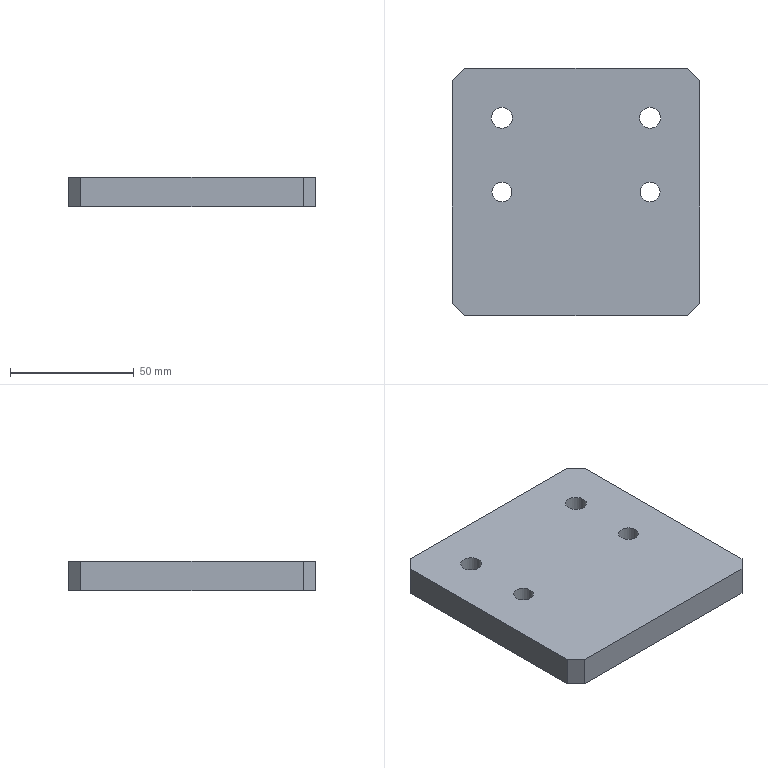Part | NX | features BREP 1 | 1 solid | 14 faces | box 100 x 100 x 12 mm | volume 116832 mm3 | plane 10 | cylinder 4 | commonest cylinder face diameters 8 x2 8.5 x2
STEP:
#1=CARTESIAN_POINT('',(50.,45.,3.));
#2=VERTEX_POINT('',#1);
#3=CARTESIAN_POINT('',(50.,-45.,3.));
#4=VERTEX_POINT('',#3);
#5=CARTESIAN_POINT('',(50.,50.,3.));
#6=DIRECTION('',(0.,-1.,0.));
#7=VECTOR('',#6,1000.);
#8=LINE('',#5,#7);
#9=EDGE_CURVE('',#2,#4,#8,.T.);
#10=ORIENTED_EDGE('',*,*,#9,.F.);
#11=CARTESIAN_POINT('',(50.,45.,15.));
#12=VERTEX_POINT('',#11);
#13=CARTESIAN_POINT('',(50.,45.,15.));
#14=DIRECTION('',(0.,0.,1.));
#15=VECTOR('',#14,1000.);
#16=LINE('',#13,#15);
#17=EDGE_CURVE('',#2,#12,#16,.T.);
#18=ORIENTED_EDGE('',*,*,#17,.T.);
#19=CARTESIAN_POINT('',(50.,-45.,15.));
#20=VERTEX_POINT('',#19);
#21=CARTESIAN_POINT('',(50.,50.,15.));
#22=DIRECTION('',(0.,1.,0.));
#23=VECTOR('',#22,1000.);
#24=LINE('',#21,#23);
#25=EDGE_CURVE('',#20,#12,#24,.T.);
#26=ORIENTED_EDGE('',*,*,#25,.F.);
#27=CARTESIAN_POINT('',(50.,-45.,15.));
#28=DIRECTION('',(0.,0.,-1.));
#29=VECTOR('',#28,1000.);
#30=LINE('',#27,#29);
#31=EDGE_CURVE('',#20,#4,#30,.T.);
#32=ORIENTED_EDGE('',*,*,#31,.T.);
#33=EDGE_LOOP('',(#10,#18,#26,#32));
#34=FACE_BOUND('',#33,.T.);
#35=CARTESIAN_POINT('',(50.,50.,15.));
#36=DIRECTION('',(-1.,0.,0.));
#37=DIRECTION('',(0.,0.,-1.));
#38=AXIS2_PLACEMENT_3D('',#35,#36,#37);
#39=PLANE('',#38);
#40=ADVANCED_FACE('',(#34),#39,.F.);
#41=CARTESIAN_POINT('',(45.,50.,3.));
#42=VERTEX_POINT('',#41);
#43=CARTESIAN_POINT('',(-45.,50.,3.));
#44=VERTEX_POINT('',#43);
#45=CARTESIAN_POINT('',(570.,50.,3.));
#46=DIRECTION('',(-1.,0.,0.));
#47=VECTOR('',#46,1000.);
#48=LINE('',#45,#47);
#49=EDGE_CURVE('',#42,#44,#48,.T.);
#50=ORIENTED_EDGE('',*,*,#49,.T.);
#51=CARTESIAN_POINT('',(-45.,50.,15.));
#52=VERTEX_POINT('',#51);
#53=CARTESIAN_POINT('',(-45.,50.,15.));
#54=DIRECTION('',(0.,0.,1.));
#55=VECTOR('',#54,1000.);
#56=LINE('',#53,#55);
#57=EDGE_CURVE('',#44,#52,#56,.T.);
#58=ORIENTED_EDGE('',*,*,#57,.T.);
#59=CARTESIAN_POINT('',(45.,50.,15.));
#60=VERTEX_POINT('',#59);
#61=CARTESIAN_POINT('',(-50.,50.,15.));
#62=DIRECTION('',(-1.,0.,0.));
#63=VECTOR('',#62,1000.);
#64=LINE('',#61,#63);
#65=EDGE_CURVE('',#60,#52,#64,.T.);
#66=ORIENTED_EDGE('',*,*,#65,.F.);
#67=CARTESIAN_POINT('',(45.,50.,15.));
#68=DIRECTION('',(0.,0.,-1.));
#69=VECTOR('',#68,1000.);
#70=LINE('',#67,#69);
#71=EDGE_CURVE('',#60,#42,#70,.T.);
#72=ORIENTED_EDGE('',*,*,#71,.T.);
#73=EDGE_LOOP('',(#50,#58,#66,#72));
#74=FACE_BOUND('',#73,.T.);
#75=CARTESIAN_POINT('',(-50.,50.,15.));
#76=DIRECTION('',(0.,-1.,0.));
#77=DIRECTION('',(0.,0.,1.));
#78=AXIS2_PLACEMENT_3D('',#75,#76,#77);
#79=PLANE('',#78);
#80=ADVANCED_FACE('',(#74),#79,.F.);
#81=CARTESIAN_POINT('',(-50.,-45.,3.));
#82=VERTEX_POINT('',#81);
#83=CARTESIAN_POINT('',(-50.,45.,3.));
#84=VERTEX_POINT('',#83);
#85=CARTESIAN_POINT('',(-50.,50.,3.));
#86=DIRECTION('',(0.,1.,0.));
#87=VECTOR('',#86,1000.);
#88=LINE('',#85,#87);
#89=EDGE_CURVE('',#82,#84,#88,.T.);
#90=ORIENTED_EDGE('',*,*,#89,.F.);
#91=CARTESIAN_POINT('',(-50.,-45.,15.));
#92=VERTEX_POINT('',#91);
#93=CARTESIAN_POINT('',(-50.,-45.,15.));
#94=DIRECTION('',(0.,0.,1.));
#95=VECTOR('',#94,1000.);
#96=LINE('',#93,#95);
#97=EDGE_CURVE('',#82,#92,#96,.T.);
#98=ORIENTED_EDGE('',*,*,#97,.T.);
#99=CARTESIAN_POINT('',(-50.,45.,15.));
#100=VERTEX_POINT('',#99);
#101=CARTESIAN_POINT('',(-50.,50.,15.));
#102=DIRECTION('',(0.,-1.,0.));
#103=VECTOR('',#102,1000.);
#104=LINE('',#101,#103);
#105=EDGE_CURVE('',#100,#92,#104,.T.);
#106=ORIENTED_EDGE('',*,*,#105,.F.);
#107=CARTESIAN_POINT('',(-50.,45.,15.));
#108=DIRECTION('',(0.,0.,-1.));
#109=VECTOR('',#108,1000.);
#110=LINE('',#107,#109);
#111=EDGE_CURVE('',#100,#84,#110,.T.);
#112=ORIENTED_EDGE('',*,*,#111,.T.);
#113=EDGE_LOOP('',(#90,#98,#106,#112));
#114=FACE_BOUND('',#113,.T.);
#115=CARTESIAN_POINT('',(-50.,50.,15.));
#116=DIRECTION('',(1.,0.,0.));
#117=DIRECTION('',(0.,-1.,0.));
#118=AXIS2_PLACEMENT_3D('',#115,#116,#117);
#119=PLANE('',#118);
#120=ADVANCED_FACE('',(#114),#119,.F.);
#121=CARTESIAN_POINT('',(45.,-50.,3.));
#122=VERTEX_POINT('',#121);
#123=CARTESIAN_POINT('',(-45.,-50.,3.));
#124=VERTEX_POINT('',#123);
#125=CARTESIAN_POINT('',(-50.,-50.,3.));
#126=DIRECTION('',(-1.,0.,0.));
#127=VECTOR('',#126,1000.);
#128=LINE('',#125,#127);
#129=EDGE_CURVE('',#122,#124,#128,.T.);
#130=ORIENTED_EDGE('',*,*,#129,.F.);
#131=CARTESIAN_POINT('',(45.,-50.,15.));
#132=VERTEX_POINT('',#131);
#133=CARTESIAN_POINT('',(45.,-50.,15.));
#134=DIRECTION('',(0.,0.,1.));
#135=VECTOR('',#134,1000.);
#136=LINE('',#133,#135);
#137=EDGE_CURVE('',#122,#132,#136,.T.);
#138=ORIENTED_EDGE('',*,*,#137,.T.);
#139=CARTESIAN_POINT('',(-45.,-50.,15.));
#140=VERTEX_POINT('',#139);
#141=CARTESIAN_POINT('',(-50.,-50.,15.));
#142=DIRECTION('',(1.,0.,0.));
#143=VECTOR('',#142,1000.);
#144=LINE('',#141,#143);
#145=EDGE_CURVE('',#140,#132,#144,.T.);
#146=ORIENTED_EDGE('',*,*,#145,.F.);
#147=CARTESIAN_POINT('',(-45.,-50.,15.));
#148=DIRECTION('',(0.,0.,-1.));
#149=VECTOR('',#148,1000.);
#150=LINE('',#147,#149);
#151=EDGE_CURVE('',#140,#124,#150,.T.);
#152=ORIENTED_EDGE('',*,*,#151,.T.);
#153=EDGE_LOOP('',(#130,#138,#146,#152));
#154=FACE_BOUND('',#153,.T.);
#155=CARTESIAN_POINT('',(-50.,-50.,15.));
#156=DIRECTION('',(0.,1.,0.));
#157=DIRECTION('',(0.,0.,-1.));
#158=AXIS2_PLACEMENT_3D('',#155,#156,#157);
#159=PLANE('',#158);
#160=ADVANCED_FACE('',(#154),#159,.F.);
#161=ORIENTED_EDGE('',*,*,#97,.F.);
#162=CARTESIAN_POINT('',(-45.,-50.,3.));
#163=DIRECTION('',(0.7071,-0.7071,0.));
#164=VECTOR('',#163,1000.);
#165=LINE('',#162,#164);
#166=EDGE_CURVE('',#82,#124,#165,.T.);
#167=ORIENTED_EDGE('',*,*,#166,.T.);
#168=ORIENTED_EDGE('',*,*,#151,.F.);
#169=CARTESIAN_POINT('',(-47.5,-47.5,15.));
#170=DIRECTION('',(0.7071,-0.7071,0.));
#171=VECTOR('',#170,1000.);
#172=LINE('',#169,#171);
#173=EDGE_CURVE('',#92,#140,#172,.T.);
#174=ORIENTED_EDGE('',*,*,#173,.F.);
#175=EDGE_LOOP('',(#161,#167,#168,#174));
#176=FACE_BOUND('',#175,.T.);
#177=CARTESIAN_POINT('',(-45.,-50.,15.));
#178=DIRECTION('',(0.7071,0.7071,0.));
#179=DIRECTION('',(0.,0.,1.));
#180=AXIS2_PLACEMENT_3D('',#177,#178,#179);
#181=PLANE('',#180);
#182=ADVANCED_FACE('',(#176),#181,.F.);
#183=ORIENTED_EDGE('',*,*,#137,.F.);
#184=CARTESIAN_POINT('',(50.,-45.,3.));
#185=DIRECTION('',(0.7071,0.7071,0.));
#186=VECTOR('',#185,1000.);
#187=LINE('',#184,#186);
#188=EDGE_CURVE('',#122,#4,#187,.T.);
#189=ORIENTED_EDGE('',*,*,#188,.T.);
#190=ORIENTED_EDGE('',*,*,#31,.F.);
#191=CARTESIAN_POINT('',(47.5,-47.5,15.));
#192=DIRECTION('',(0.7071,0.7071,0.));
#193=VECTOR('',#192,1000.);
#194=LINE('',#191,#193);
#195=EDGE_CURVE('',#132,#20,#194,.T.);
#196=ORIENTED_EDGE('',*,*,#195,.F.);
#197=EDGE_LOOP('',(#183,#189,#190,#196));
#198=FACE_BOUND('',#197,.T.);
#199=CARTESIAN_POINT('',(50.,-45.,15.));
#200=DIRECTION('',(-0.7071,0.7071,0.));
#201=DIRECTION('',(0.,0.,1.));
#202=AXIS2_PLACEMENT_3D('',#199,#200,#201);
#203=PLANE('',#202);
#204=ADVANCED_FACE('',(#198),#203,.F.);
#205=ORIENTED_EDGE('',*,*,#17,.F.);
#206=CARTESIAN_POINT('',(45.,50.,3.));
#207=DIRECTION('',(-0.7071,0.7071,0.));
#208=VECTOR('',#207,1000.);
#209=LINE('',#206,#208);
#210=EDGE_CURVE('',#2,#42,#209,.T.);
#211=ORIENTED_EDGE('',*,*,#210,.T.);
#212=ORIENTED_EDGE('',*,*,#71,.F.);
#213=CARTESIAN_POINT('',(47.5,47.5,15.));
#214=DIRECTION('',(-0.7071,0.7071,0.));
#215=VECTOR('',#214,1000.);
#216=LINE('',#213,#215);
#217=EDGE_CURVE('',#12,#60,#216,.T.);
#218=ORIENTED_EDGE('',*,*,#217,.F.);
#219=EDGE_LOOP('',(#205,#211,#212,#218));
#220=FACE_BOUND('',#219,.T.);
#221=CARTESIAN_POINT('',(45.,50.,15.));
#222=DIRECTION('',(-0.7071,-0.7071,0.));
#223=DIRECTION('',(0.,0.,1.));
#224=AXIS2_PLACEMENT_3D('',#221,#222,#223);
#225=PLANE('',#224);
#226=ADVANCED_FACE('',(#220),#225,.F.);
#227=ORIENTED_EDGE('',*,*,#57,.F.);
#228=CARTESIAN_POINT('',(-50.,45.,3.));
#229=DIRECTION('',(-0.7071,-0.7071,0.));
#230=VECTOR('',#229,1000.);
#231=LINE('',#228,#230);
#232=EDGE_CURVE('',#44,#84,#231,.T.);
#233=ORIENTED_EDGE('',*,*,#232,.T.);
#234=ORIENTED_EDGE('',*,*,#111,.F.);
#235=CARTESIAN_POINT('',(-47.5,47.5,15.));
#236=DIRECTION('',(-0.7071,-0.7071,0.));
#237=VECTOR('',#236,1000.);
#238=LINE('',#235,#237);
#239=EDGE_CURVE('',#52,#100,#238,.T.);
#240=ORIENTED_EDGE('',*,*,#239,.F.);
#241=EDGE_LOOP('',(#227,#233,#234,#240));
#242=FACE_BOUND('',#241,.T.);
#243=CARTESIAN_POINT('',(-50.,45.,15.));
#244=DIRECTION('',(0.7071,-0.7071,0.));
#245=DIRECTION('',(0.,0.,1.));
#246=AXIS2_PLACEMENT_3D('',#243,#244,#245);
#247=PLANE('',#246);
#248=ADVANCED_FACE('',(#242),#247,.F.);
#249=CARTESIAN_POINT('',(34.25,30.,15.));
#250=VERTEX_POINT('',#249);
#251=CARTESIAN_POINT('',(30.,30.,15.));
#252=DIRECTION('',(0.,0.,1.));
#253=DIRECTION('',(1.,0.,0.));
#254=AXIS2_PLACEMENT_3D('',#251,#252,#253);
#255=CIRCLE('',#254,4.25);
#256=EDGE_CURVE('',#250,#250,#255,.T.);
#257=ORIENTED_EDGE('',*,*,#256,.F.);
#258=EDGE_LOOP('',(#257));
#259=FACE_BOUND('',#258,.T.);
#260=CARTESIAN_POINT('',(-25.75,30.,15.));
#261=VERTEX_POINT('',#260);
#262=CARTESIAN_POINT('',(-30.,30.,15.));
#263=DIRECTION('',(0.,0.,1.));
#264=DIRECTION('',(1.,0.,0.));
#265=AXIS2_PLACEMENT_3D('',#262,#263,#264);
#266=CIRCLE('',#265,4.25);
#267=EDGE_CURVE('',#261,#261,#266,.T.);
#268=ORIENTED_EDGE('',*,*,#267,.F.);
#269=EDGE_LOOP('',(#268));
#270=FACE_BOUND('',#269,.T.);
#271=CARTESIAN_POINT('',(34.,0.,15.));
#272=VERTEX_POINT('',#271);
#273=CARTESIAN_POINT('',(30.,0.,15.));
#274=DIRECTION('',(0.,0.,1.));
#275=DIRECTION('',(1.,0.,0.));
#276=AXIS2_PLACEMENT_3D('',#273,#274,#275);
#277=CIRCLE('',#276,4.);
#278=EDGE_CURVE('',#272,#272,#277,.T.);
#279=ORIENTED_EDGE('',*,*,#278,.F.);
#280=EDGE_LOOP('',(#279));
#281=FACE_BOUND('',#280,.T.);
#282=CARTESIAN_POINT('',(-26.,0.,15.));
#283=VERTEX_POINT('',#282);
#284=CARTESIAN_POINT('',(-30.,0.,15.));
#285=DIRECTION('',(0.,0.,1.));
#286=DIRECTION('',(1.,0.,0.));
#287=AXIS2_PLACEMENT_3D('',#284,#285,#286);
#288=CIRCLE('',#287,4.);
#289=EDGE_CURVE('',#283,#283,#288,.T.);
#290=ORIENTED_EDGE('',*,*,#289,.F.);
#291=EDGE_LOOP('',(#290));
#292=FACE_BOUND('',#291,.T.);
#293=ORIENTED_EDGE('',*,*,#105,.T.);
#294=ORIENTED_EDGE('',*,*,#173,.T.);
#295=ORIENTED_EDGE('',*,*,#145,.T.);
#296=ORIENTED_EDGE('',*,*,#195,.T.);
#297=ORIENTED_EDGE('',*,*,#25,.T.);
#298=ORIENTED_EDGE('',*,*,#217,.T.);
#299=ORIENTED_EDGE('',*,*,#65,.T.);
#300=ORIENTED_EDGE('',*,*,#239,.T.);
#301=EDGE_LOOP('',(#293,#294,#295,#296,#297,#298,#299,#300));
#302=FACE_BOUND('',#301,.T.);
#303=CARTESIAN_POINT('',(0.,0.,15.));
#304=DIRECTION('',(0.,0.,1.));
#305=DIRECTION('',(-1.,0.,0.));
#306=AXIS2_PLACEMENT_3D('',#303,#304,#305);
#307=PLANE('',#306);
#308=ADVANCED_FACE('',(#259,#270,#281,#292,#302),#307,.T.);
#309=CARTESIAN_POINT('',(25.75,30.,3.));
#310=VERTEX_POINT('',#309);
#311=CARTESIAN_POINT('',(30.,30.,3.));
#312=DIRECTION('',(0.,0.,-1.));
#313=DIRECTION('',(-1.,0.,0.));
#314=AXIS2_PLACEMENT_3D('',#311,#312,#313);
#315=CIRCLE('',#314,4.25);
#316=EDGE_CURVE('',#310,#310,#315,.T.);
#317=ORIENTED_EDGE('',*,*,#316,.F.);
#318=EDGE_LOOP('',(#317));
#319=FACE_BOUND('',#318,.T.);
#320=CARTESIAN_POINT('',(-34.25,30.,3.));
#321=VERTEX_POINT('',#320);
#322=CARTESIAN_POINT('',(-30.,30.,3.));
#323=DIRECTION('',(0.,0.,-1.));
#324=DIRECTION('',(-1.,0.,0.));
#325=AXIS2_PLACEMENT_3D('',#322,#323,#324);
#326=CIRCLE('',#325,4.25);
#327=EDGE_CURVE('',#321,#321,#326,.T.);
#328=ORIENTED_EDGE('',*,*,#327,.F.);
#329=EDGE_LOOP('',(#328));
#330=FACE_BOUND('',#329,.T.);
#331=CARTESIAN_POINT('',(26.,0.,3.));
#332=VERTEX_POINT('',#331);
#333=CARTESIAN_POINT('',(30.,0.,3.));
#334=DIRECTION('',(0.,0.,-1.));
#335=DIRECTION('',(-1.,0.,0.));
#336=AXIS2_PLACEMENT_3D('',#333,#334,#335);
#337=CIRCLE('',#336,4.);
#338=EDGE_CURVE('',#332,#332,#337,.T.);
#339=ORIENTED_EDGE('',*,*,#338,.F.);
#340=EDGE_LOOP('',(#339));
#341=FACE_BOUND('',#340,.T.);
#342=CARTESIAN_POINT('',(-34.,0.,3.));
#343=VERTEX_POINT('',#342);
#344=CARTESIAN_POINT('',(-30.,0.,3.));
#345=DIRECTION('',(0.,0.,-1.));
#346=DIRECTION('',(-1.,0.,0.));
#347=AXIS2_PLACEMENT_3D('',#344,#345,#346);
#348=CIRCLE('',#347,4.);
#349=EDGE_CURVE('',#343,#343,#348,.T.);
#350=ORIENTED_EDGE('',*,*,#349,.F.);
#351=EDGE_LOOP('',(#350));
#352=FACE_BOUND('',#351,.T.);
#353=ORIENTED_EDGE('',*,*,#9,.T.);
#354=ORIENTED_EDGE('',*,*,#188,.F.);
#355=ORIENTED_EDGE('',*,*,#129,.T.);
#356=ORIENTED_EDGE('',*,*,#166,.F.);
#357=ORIENTED_EDGE('',*,*,#89,.T.);
#358=ORIENTED_EDGE('',*,*,#232,.F.);
#359=ORIENTED_EDGE('',*,*,#49,.F.);
#360=ORIENTED_EDGE('',*,*,#210,.F.);
#361=EDGE_LOOP('',(#353,#354,#355,#356,#357,#358,#359,#360));
#362=FACE_BOUND('',#361,.T.);
#363=CARTESIAN_POINT('',(-380.,-300.,3.));
#364=DIRECTION('',(0.,0.,-1.));
#365=DIRECTION('',(1.,0.,0.));
#366=AXIS2_PLACEMENT_3D('',#363,#364,#365);
#367=PLANE('',#366);
#368=ADVANCED_FACE('',(#319,#330,#341,#352,#362),#367,.T.);
#369=ORIENTED_EDGE('',*,*,#289,.T.);
#370=EDGE_LOOP('',(#369));
#371=FACE_BOUND('',#370,.T.);
#372=ORIENTED_EDGE('',*,*,#349,.T.);
#373=EDGE_LOOP('',(#372));
#374=FACE_BOUND('',#373,.T.);
#375=CARTESIAN_POINT('',(-30.,0.,3.));
#376=DIRECTION('',(0.,0.,-1.));
#377=DIRECTION('',(1.,0.,0.));
#378=AXIS2_PLACEMENT_3D('',#375,#376,#377);
#379=CYLINDRICAL_SURFACE('',#378,4.);
#380=ADVANCED_FACE('',(#371,#374),#379,.F.);
#381=ORIENTED_EDGE('',*,*,#278,.T.);
#382=EDGE_LOOP('',(#381));
#383=FACE_BOUND('',#382,.T.);
#384=ORIENTED_EDGE('',*,*,#338,.T.);
#385=EDGE_LOOP('',(#384));
#386=FACE_BOUND('',#385,.T.);
#387=CARTESIAN_POINT('',(30.,0.,3.));
#388=DIRECTION('',(0.,0.,-1.));
#389=DIRECTION('',(1.,0.,0.));
#390=AXIS2_PLACEMENT_3D('',#387,#388,#389);
#391=CYLINDRICAL_SURFACE('',#390,4.);
#392=ADVANCED_FACE('',(#383,#386),#391,.F.);
#393=ORIENTED_EDGE('',*,*,#267,.T.);
#394=EDGE_LOOP('',(#393));
#395=FACE_BOUND('',#394,.T.);
#396=ORIENTED_EDGE('',*,*,#327,.T.);
#397=EDGE_LOOP('',(#396));
#398=FACE_BOUND('',#397,.T.);
#399=CARTESIAN_POINT('',(-30.,30.,3.));
#400=DIRECTION('',(0.,0.,-1.));
#401=DIRECTION('',(1.,0.,0.));
#402=AXIS2_PLACEMENT_3D('',#399,#400,#401);
#403=CYLINDRICAL_SURFACE('',#402,4.25);
#404=ADVANCED_FACE('',(#395,#398),#403,.F.);
#405=ORIENTED_EDGE('',*,*,#256,.T.);
#406=EDGE_LOOP('',(#405));
#407=FACE_BOUND('',#406,.T.);
#408=ORIENTED_EDGE('',*,*,#316,.T.);
#409=EDGE_LOOP('',(#408));
#410=FACE_BOUND('',#409,.T.);
#411=CARTESIAN_POINT('',(30.,30.,3.));
#412=DIRECTION('',(0.,0.,-1.));
#413=DIRECTION('',(1.,0.,0.));
#414=AXIS2_PLACEMENT_3D('',#411,#412,#413);
#415=CYLINDRICAL_SURFACE('',#414,4.25);
#416=ADVANCED_FACE('',(#407,#410),#415,.F.);
#417=CLOSED_SHELL('',(#40,#80,#120,#160,#182,#204,#226,#248,#308,#368,#380,#392,#404,#416));
#418=MANIFOLD_SOLID_BREP('',#417);
#419=(LENGTH_UNIT()NAMED_UNIT(*)SI_UNIT(.MILLI.,.METRE.));
#420=UNCERTAINTY_MEASURE_WITH_UNIT(LENGTH_MEASURE(0.00001),#419,'','');
#421=(NAMED_UNIT(*)PLANE_ANGLE_UNIT()SI_UNIT($,.RADIAN.));
#422=(NAMED_UNIT(*)SI_UNIT($,.STERADIAN.)SOLID_ANGLE_UNIT());
#423=(GEOMETRIC_REPRESENTATION_CONTEXT(3)GLOBAL_UNCERTAINTY_ASSIGNED_CONTEXT((#420))GLOBAL_UNIT_ASSIGNED_CONTEXT((#419,#421,#422))REPRESENTATION_CONTEXT('',''));
#424=ADVANCED_BREP_SHAPE_REPRESENTATION('',(#418),#423);